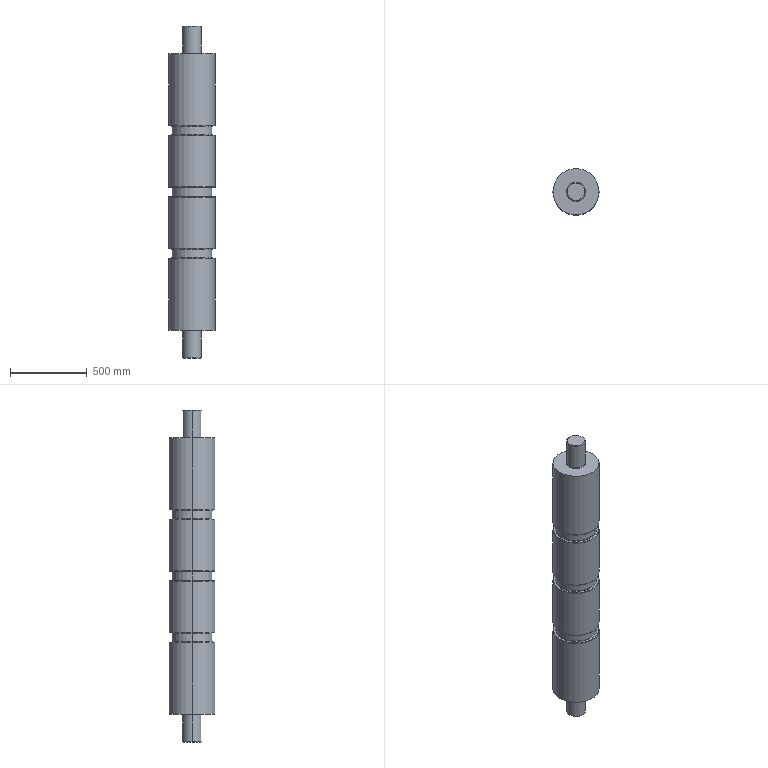Part | SolidWorks | features Chamfer 2, ICE 2, Extrusion 1, Fillet 1, LPattern 1, RefAxis 1, RevCut 1 | 1 solid | 60 faces | box 300 x 300 x 2160 mm | volume 128138036 mm3 | torus 24 | cylinder 18 | plane 10 | cone 8 | commonest cylinder face diameters 300 x8 260 x6 120 x4
STEP:
#1=CARTESIAN_POINT('',(-57.,0.,-180.));
#2=VERTEX_POINT('',#1);
#3=CARTESIAN_POINT('',(57.,0.,-180.));
#4=VERTEX_POINT('',#3);
#5=CARTESIAN_POINT('',(0.,0.,-180.));
#6=DIRECTION('',(0.,0.,-1.));
#7=DIRECTION('',(-1.,0.,0.));
#8=AXIS2_PLACEMENT_3D('',#5,#6,#7);
#9=CIRCLE('',#8,57.);
#10=EDGE_CURVE('',#2,#4,#9,.T.);
#11=ORIENTED_EDGE('',*,*,#10,.F.);
#12=CARTESIAN_POINT('',(-60.,0.,-177.));
#13=VERTEX_POINT('',#12);
#14=CARTESIAN_POINT('',(-57.,0.,-180.));
#15=DIRECTION('',(-0.7071,0.,0.7071));
#16=VECTOR('',#15,1000.);
#17=LINE('',#14,#16);
#18=EDGE_CURVE('',#2,#13,#17,.T.);
#19=ORIENTED_EDGE('',*,*,#18,.T.);
#20=CARTESIAN_POINT('',(60.,0.,-177.));
#21=VERTEX_POINT('',#20);
#22=CARTESIAN_POINT('',(0.,0.,-177.));
#23=DIRECTION('',(0.,0.,1.));
#24=DIRECTION('',(-1.,0.,0.));
#25=AXIS2_PLACEMENT_3D('',#22,#23,#24);
#26=CIRCLE('',#25,60.);
#27=EDGE_CURVE('',#21,#13,#26,.T.);
#28=ORIENTED_EDGE('',*,*,#27,.F.);
#29=CARTESIAN_POINT('',(57.,0.,-180.));
#30=DIRECTION('',(0.7071,0.,0.7071));
#31=VECTOR('',#30,1000.);
#32=LINE('',#29,#31);
#33=EDGE_CURVE('',#4,#21,#32,.T.);
#34=ORIENTED_EDGE('',*,*,#33,.F.);
#35=EDGE_LOOP('',(#11,#19,#28,#34));
#36=FACE_OUTER_BOUND('',#35,.T.);
#37=CARTESIAN_POINT('',(0.,0.,-180.));
#38=DIRECTION('',(0.,0.,1.));
#39=DIRECTION('',(1.,0.,0.));
#40=AXIS2_PLACEMENT_3D('',#37,#38,#39);
#41=CONICAL_SURFACE('',#40,57.,0.7854);
#42=ADVANCED_FACE('',(#36),#41,.T.);
#43=CARTESIAN_POINT('',(-60.,0.,-3.));
#44=VERTEX_POINT('',#43);
#45=CARTESIAN_POINT('',(60.,0.,-3.));
#46=VERTEX_POINT('',#45);
#47=CARTESIAN_POINT('',(0.,0.,-3.));
#48=DIRECTION('',(0.,0.,-1.));
#49=DIRECTION('',(1.,0.,0.));
#50=AXIS2_PLACEMENT_3D('',#47,#48,#49);
#51=CIRCLE('',#50,60.);
#52=EDGE_CURVE('',#44,#46,#51,.T.);
#53=ORIENTED_EDGE('',*,*,#52,.F.);
#54=CARTESIAN_POINT('',(-63.,0.,0.));
#55=VERTEX_POINT('',#54);
#56=CARTESIAN_POINT('',(-60.,0.,-3.));
#57=DIRECTION('',(-0.7071,0.,0.7071));
#58=VECTOR('',#57,1000.);
#59=LINE('',#56,#58);
#60=EDGE_CURVE('',#44,#55,#59,.T.);
#61=ORIENTED_EDGE('',*,*,#60,.T.);
#62=CARTESIAN_POINT('',(63.,0.,0.));
#63=VERTEX_POINT('',#62);
#64=CARTESIAN_POINT('',(0.,0.,0.));
#65=DIRECTION('',(0.,0.,1.));
#66=DIRECTION('',(1.,0.,0.));
#67=AXIS2_PLACEMENT_3D('',#64,#65,#66);
#68=CIRCLE('',#67,63.);
#69=EDGE_CURVE('',#63,#55,#68,.T.);
#70=ORIENTED_EDGE('',*,*,#69,.F.);
#71=CARTESIAN_POINT('',(60.,0.,-3.));
#72=DIRECTION('',(0.7071,0.,0.7071));
#73=VECTOR('',#72,1000.);
#74=LINE('',#71,#73);
#75=EDGE_CURVE('',#46,#63,#74,.T.);
#76=ORIENTED_EDGE('',*,*,#75,.F.);
#77=EDGE_LOOP('',(#53,#61,#70,#76));
#78=FACE_OUTER_BOUND('',#77,.T.);
#79=CARTESIAN_POINT('',(0.,0.,-3.));
#80=DIRECTION('',(0.,0.,1.));
#81=DIRECTION('',(1.,0.,0.));
#82=AXIS2_PLACEMENT_3D('',#79,#80,#81);
#83=CONICAL_SURFACE('',#82,60.,0.7854);
#84=ADVANCED_FACE('',(#78),#83,.T.);
#85=ORIENTED_EDGE('',*,*,#27,.T.);
#86=CARTESIAN_POINT('',(-60.,0.,-180.));
#87=DIRECTION('',(0.,0.,1.));
#88=VECTOR('',#87,1000.);
#89=LINE('',#86,#88);
#90=EDGE_CURVE('',#13,#44,#89,.T.);
#91=ORIENTED_EDGE('',*,*,#90,.T.);
#92=ORIENTED_EDGE('',*,*,#52,.T.);
#93=CARTESIAN_POINT('',(60.,0.,-180.));
#94=DIRECTION('',(0.,0.,1.));
#95=VECTOR('',#94,1000.);
#96=LINE('',#93,#95);
#97=EDGE_CURVE('',#21,#46,#96,.T.);
#98=ORIENTED_EDGE('',*,*,#97,.F.);
#99=EDGE_LOOP('',(#85,#91,#92,#98));
#100=FACE_OUTER_BOUND('',#99,.T.);
#101=CARTESIAN_POINT('',(0.,0.,-180.));
#102=DIRECTION('',(0.,0.,1.));
#103=DIRECTION('',(1.,0.,0.));
#104=AXIS2_PLACEMENT_3D('',#101,#102,#103);
#105=CYLINDRICAL_SURFACE('',#104,60.);
#106=ADVANCED_FACE('',(#100),#105,.T.);
#107=CARTESIAN_POINT('',(57.,0.,1980.));
#108=VERTEX_POINT('',#107);
#109=CARTESIAN_POINT('',(-57.,0.,1980.));
#110=VERTEX_POINT('',#109);
#111=CARTESIAN_POINT('',(0.,0.,1980.));
#112=DIRECTION('',(0.,0.,1.));
#113=DIRECTION('',(1.,0.,0.));
#114=AXIS2_PLACEMENT_3D('',#111,#112,#113);
#115=CIRCLE('',#114,57.);
#116=EDGE_CURVE('',#108,#110,#115,.T.);
#117=ORIENTED_EDGE('',*,*,#116,.F.);
#118=CARTESIAN_POINT('',(60.,0.,1977.));
#119=VERTEX_POINT('',#118);
#120=CARTESIAN_POINT('',(57.,0.,1980.));
#121=DIRECTION('',(0.7071,0.,-0.7071));
#122=VECTOR('',#121,1000.);
#123=LINE('',#120,#122);
#124=EDGE_CURVE('',#108,#119,#123,.T.);
#125=ORIENTED_EDGE('',*,*,#124,.T.);
#126=CARTESIAN_POINT('',(-60.,0.,1977.));
#127=VERTEX_POINT('',#126);
#128=CARTESIAN_POINT('',(0.,0.,1977.));
#129=DIRECTION('',(0.,0.,-1.));
#130=DIRECTION('',(1.,0.,0.));
#131=AXIS2_PLACEMENT_3D('',#128,#129,#130);
#132=CIRCLE('',#131,60.);
#133=EDGE_CURVE('',#127,#119,#132,.T.);
#134=ORIENTED_EDGE('',*,*,#133,.F.);
#135=CARTESIAN_POINT('',(-57.,0.,1980.));
#136=DIRECTION('',(-0.7071,0.,-0.7071));
#137=VECTOR('',#136,1000.);
#138=LINE('',#135,#137);
#139=EDGE_CURVE('',#110,#127,#138,.T.);
#140=ORIENTED_EDGE('',*,*,#139,.F.);
#141=EDGE_LOOP('',(#117,#125,#134,#140));
#142=FACE_OUTER_BOUND('',#141,.T.);
#143=CARTESIAN_POINT('',(0.,0.,1980.));
#144=DIRECTION('',(0.,0.,-1.));
#145=DIRECTION('',(-1.,0.,0.));
#146=AXIS2_PLACEMENT_3D('',#143,#144,#145);
#147=CONICAL_SURFACE('',#146,57.,0.7854);
#148=ADVANCED_FACE('',(#142),#147,.T.);
#149=CARTESIAN_POINT('',(60.,0.,1803.));
#150=VERTEX_POINT('',#149);
#151=CARTESIAN_POINT('',(-60.,0.,1803.));
#152=VERTEX_POINT('',#151);
#153=CARTESIAN_POINT('',(0.,0.,1803.));
#154=DIRECTION('',(0.,0.,1.));
#155=DIRECTION('',(1.,0.,0.));
#156=AXIS2_PLACEMENT_3D('',#153,#154,#155);
#157=CIRCLE('',#156,60.);
#158=EDGE_CURVE('',#150,#152,#157,.T.);
#159=ORIENTED_EDGE('',*,*,#158,.F.);
#160=CARTESIAN_POINT('',(63.,0.,1800.));
#161=VERTEX_POINT('',#160);
#162=CARTESIAN_POINT('',(60.,0.,1803.));
#163=DIRECTION('',(0.7071,0.,-0.7071));
#164=VECTOR('',#163,1000.);
#165=LINE('',#162,#164);
#166=EDGE_CURVE('',#150,#161,#165,.T.);
#167=ORIENTED_EDGE('',*,*,#166,.T.);
#168=CARTESIAN_POINT('',(-63.,0.,1800.));
#169=VERTEX_POINT('',#168);
#170=CARTESIAN_POINT('',(0.,0.,1800.));
#171=DIRECTION('',(0.,0.,-1.));
#172=DIRECTION('',(1.,0.,0.));
#173=AXIS2_PLACEMENT_3D('',#170,#171,#172);
#174=CIRCLE('',#173,63.);
#175=EDGE_CURVE('',#169,#161,#174,.T.);
#176=ORIENTED_EDGE('',*,*,#175,.F.);
#177=CARTESIAN_POINT('',(-60.,0.,1803.));
#178=DIRECTION('',(-0.7071,0.,-0.7071));
#179=VECTOR('',#178,1000.);
#180=LINE('',#177,#179);
#181=EDGE_CURVE('',#152,#169,#180,.T.);
#182=ORIENTED_EDGE('',*,*,#181,.F.);
#183=EDGE_LOOP('',(#159,#167,#176,#182));
#184=FACE_OUTER_BOUND('',#183,.T.);
#185=CARTESIAN_POINT('',(0.,0.,1803.));
#186=DIRECTION('',(0.,0.,-1.));
#187=DIRECTION('',(-1.,0.,0.));
#188=AXIS2_PLACEMENT_3D('',#185,#186,#187);
#189=CONICAL_SURFACE('',#188,60.,0.7854);
#190=ADVANCED_FACE('',(#184),#189,.T.);
#191=ORIENTED_EDGE('',*,*,#133,.T.);
#192=CARTESIAN_POINT('',(60.,0.,1980.));
#193=DIRECTION('',(0.,0.,-1.));
#194=VECTOR('',#193,1000.);
#195=LINE('',#192,#194);
#196=EDGE_CURVE('',#119,#150,#195,.T.);
#197=ORIENTED_EDGE('',*,*,#196,.T.);
#198=ORIENTED_EDGE('',*,*,#158,.T.);
#199=CARTESIAN_POINT('',(-60.,0.,1980.));
#200=DIRECTION('',(0.,0.,-1.));
#201=VECTOR('',#200,1000.);
#202=LINE('',#199,#201);
#203=EDGE_CURVE('',#127,#152,#202,.T.);
#204=ORIENTED_EDGE('',*,*,#203,.F.);
#205=EDGE_LOOP('',(#191,#197,#198,#204));
#206=FACE_OUTER_BOUND('',#205,.T.);
#207=CARTESIAN_POINT('',(0.,0.,1980.));
#208=DIRECTION('',(0.,0.,-1.));
#209=DIRECTION('',(-1.,0.,0.));
#210=AXIS2_PLACEMENT_3D('',#207,#208,#209);
#211=CYLINDRICAL_SURFACE('',#210,60.);
#212=ADVANCED_FACE('',(#206),#211,.T.);
#213=CARTESIAN_POINT('',(-130.,0.,473.));
#214=VERTEX_POINT('',#213);
#215=CARTESIAN_POINT('',(130.,0.,473.));
#216=VERTEX_POINT('',#215);
#217=CARTESIAN_POINT('',(0.,0.,473.));
#218=DIRECTION('',(0.,0.,1.));
#219=DIRECTION('',(1.,0.,0.));
#220=AXIS2_PLACEMENT_3D('',#217,#218,#219);
#221=CIRCLE('',#220,130.);
#222=EDGE_CURVE('',#214,#216,#221,.T.);
#223=ORIENTED_EDGE('',*,*,#222,.F.);
#224=CARTESIAN_POINT('',(-133.,0.,470.));
#225=VERTEX_POINT('',#224);
#226=CARTESIAN_POINT('',(-133.,0.,473.));
#227=DIRECTION('',(0.,1.,0.));
#228=DIRECTION('',(-1.,0.,0.));
#229=AXIS2_PLACEMENT_3D('',#226,#227,#228);
#230=CIRCLE('',#229,3.);
#231=EDGE_CURVE('',#214,#225,#230,.T.);
#232=ORIENTED_EDGE('',*,*,#231,.T.);
#233=CARTESIAN_POINT('',(133.,0.,470.));
#234=VERTEX_POINT('',#233);
#235=CARTESIAN_POINT('',(0.,0.,470.));
#236=DIRECTION('',(0.,0.,-1.));
#237=DIRECTION('',(1.,0.,0.));
#238=AXIS2_PLACEMENT_3D('',#235,#236,#237);
#239=CIRCLE('',#238,133.);
#240=EDGE_CURVE('',#234,#225,#239,.T.);
#241=ORIENTED_EDGE('',*,*,#240,.F.);
#242=CARTESIAN_POINT('',(133.,0.,473.));
#243=DIRECTION('',(0.,-1.,0.));
#244=DIRECTION('',(0.,0.,-1.));
#245=AXIS2_PLACEMENT_3D('',#242,#243,#244);
#246=CIRCLE('',#245,3.);
#247=EDGE_CURVE('',#216,#234,#246,.T.);
#248=ORIENTED_EDGE('',*,*,#247,.F.);
#249=EDGE_LOOP('',(#223,#232,#241,#248));
#250=FACE_OUTER_BOUND('',#249,.T.);
#251=CARTESIAN_POINT('',(0.,0.,473.));
#252=DIRECTION('',(0.,0.,1.));
#253=DIRECTION('',(1.,0.,0.));
#254=AXIS2_PLACEMENT_3D('',#251,#252,#253);
#255=TOROIDAL_SURFACE('',#254,133.,3.);
#256=ADVANCED_FACE('',(#250),#255,.F.);
#257=CARTESIAN_POINT('',(-150.,0.,467.));
#258=VERTEX_POINT('',#257);
#259=CARTESIAN_POINT('',(150.,0.,467.));
#260=VERTEX_POINT('',#259);
#261=CARTESIAN_POINT('',(0.,0.,467.));
#262=DIRECTION('',(0.,0.,-1.));
#263=DIRECTION('',(1.,0.,0.));
#264=AXIS2_PLACEMENT_3D('',#261,#262,#263);
#265=CIRCLE('',#264,150.);
#266=EDGE_CURVE('',#258,#260,#265,.T.);
#267=ORIENTED_EDGE('',*,*,#266,.F.);
#268=CARTESIAN_POINT('',(-147.,0.,470.));
#269=VERTEX_POINT('',#268);
#270=CARTESIAN_POINT('',(-147.,0.,467.));
#271=DIRECTION('',(0.,1.,0.));
#272=DIRECTION('',(-1.,0.,0.));
#273=AXIS2_PLACEMENT_3D('',#270,#271,#272);
#274=CIRCLE('',#273,3.);
#275=EDGE_CURVE('',#258,#269,#274,.T.);
#276=ORIENTED_EDGE('',*,*,#275,.T.);
#277=CARTESIAN_POINT('',(147.,0.,470.));
#278=VERTEX_POINT('',#277);
#279=CARTESIAN_POINT('',(0.,0.,470.));
#280=DIRECTION('',(0.,0.,1.));
#281=DIRECTION('',(1.,0.,0.));
#282=AXIS2_PLACEMENT_3D('',#279,#280,#281);
#283=CIRCLE('',#282,147.);
#284=EDGE_CURVE('',#278,#269,#283,.T.);
#285=ORIENTED_EDGE('',*,*,#284,.F.);
#286=CARTESIAN_POINT('',(147.,0.,467.));
#287=DIRECTION('',(0.,-1.,0.));
#288=DIRECTION('',(0.,0.,-1.));
#289=AXIS2_PLACEMENT_3D('',#286,#287,#288);
#290=CIRCLE('',#289,3.);
#291=EDGE_CURVE('',#260,#278,#290,.T.);
#292=ORIENTED_EDGE('',*,*,#291,.F.);
#293=EDGE_LOOP('',(#267,#276,#285,#292));
#294=FACE_OUTER_BOUND('',#293,.T.);
#295=CARTESIAN_POINT('',(0.,0.,467.));
#296=DIRECTION('',(0.,0.,1.));
#297=DIRECTION('',(1.,0.,0.));
#298=AXIS2_PLACEMENT_3D('',#295,#296,#297);
#299=TOROIDAL_SURFACE('',#298,147.,3.);
#300=ADVANCED_FACE('',(#294),#299,.T.);
#301=CARTESIAN_POINT('',(150.,0.,533.));
#302=VERTEX_POINT('',#301);
#303=CARTESIAN_POINT('',(-150.,0.,533.));
#304=VERTEX_POINT('',#303);
#305=CARTESIAN_POINT('',(0.,0.,533.));
#306=DIRECTION('',(0.,0.,1.));
#307=DIRECTION('',(-1.,0.,0.));
#308=AXIS2_PLACEMENT_3D('',#305,#306,#307);
#309=CIRCLE('',#308,150.);
#310=EDGE_CURVE('',#302,#304,#309,.T.);
#311=ORIENTED_EDGE('',*,*,#310,.F.);
#312=CARTESIAN_POINT('',(147.,0.,530.));
#313=VERTEX_POINT('',#312);
#314=CARTESIAN_POINT('',(147.,0.,533.));
#315=DIRECTION('',(0.,1.,0.));
#316=DIRECTION('',(-1.,0.,0.));
#317=AXIS2_PLACEMENT_3D('',#314,#315,#316);
#318=CIRCLE('',#317,3.);
#319=EDGE_CURVE('',#302,#313,#318,.T.);
#320=ORIENTED_EDGE('',*,*,#319,.T.);
#321=CARTESIAN_POINT('',(-147.,0.,530.));
#322=VERTEX_POINT('',#321);
#323=CARTESIAN_POINT('',(0.,0.,530.));
#324=DIRECTION('',(0.,0.,-1.));
#325=DIRECTION('',(-1.,0.,0.));
#326=AXIS2_PLACEMENT_3D('',#323,#324,#325);
#327=CIRCLE('',#326,147.);
#328=EDGE_CURVE('',#322,#313,#327,.T.);
#329=ORIENTED_EDGE('',*,*,#328,.F.);
#330=CARTESIAN_POINT('',(-147.,0.,533.));
#331=DIRECTION('',(0.,-1.,0.));
#332=DIRECTION('',(0.,0.,-1.));
#333=AXIS2_PLACEMENT_3D('',#330,#331,#332);
#334=CIRCLE('',#333,3.);
#335=EDGE_CURVE('',#304,#322,#334,.T.);
#336=ORIENTED_EDGE('',*,*,#335,.F.);
#337=EDGE_LOOP('',(#311,#320,#329,#336));
#338=FACE_OUTER_BOUND('',#337,.T.);
#339=CARTESIAN_POINT('',(0.,0.,533.));
#340=DIRECTION('',(0.,0.,-1.));
#341=DIRECTION('',(-1.,0.,0.));
#342=AXIS2_PLACEMENT_3D('',#339,#340,#341);
#343=TOROIDAL_SURFACE('',#342,147.,3.);
#344=ADVANCED_FACE('',(#338),#343,.T.);
#345=CARTESIAN_POINT('',(130.,0.,527.));
#346=VERTEX_POINT('',#345);
#347=CARTESIAN_POINT('',(-130.,0.,527.));
#348=VERTEX_POINT('',#347);
#349=CARTESIAN_POINT('',(0.,0.,527.));
#350=DIRECTION('',(0.,0.,-1.));
#351=DIRECTION('',(-1.,0.,0.));
#352=AXIS2_PLACEMENT_3D('',#349,#350,#351);
#353=CIRCLE('',#352,130.);
#354=EDGE_CURVE('',#346,#348,#353,.T.);
#355=ORIENTED_EDGE('',*,*,#354,.F.);
#356=CARTESIAN_POINT('',(133.,0.,530.));
#357=VERTEX_POINT('',#356);
#358=CARTESIAN_POINT('',(133.,0.,527.));
#359=DIRECTION('',(0.,1.,0.));
#360=DIRECTION('',(-1.,0.,0.));
#361=AXIS2_PLACEMENT_3D('',#358,#359,#360);
#362=CIRCLE('',#361,3.);
#363=EDGE_CURVE('',#346,#357,#362,.T.);
#364=ORIENTED_EDGE('',*,*,#363,.T.);
#365=CARTESIAN_POINT('',(-133.,0.,530.));
#366=VERTEX_POINT('',#365);
#367=CARTESIAN_POINT('',(0.,0.,530.));
#368=DIRECTION('',(0.,0.,1.));
#369=DIRECTION('',(-1.,0.,0.));
#370=AXIS2_PLACEMENT_3D('',#367,#368,#369);
#371=CIRCLE('',#370,133.);
#372=EDGE_CURVE('',#366,#357,#371,.T.);
#373=ORIENTED_EDGE('',*,*,#372,.F.);
#374=CARTESIAN_POINT('',(-133.,0.,527.));
#375=DIRECTION('',(0.,-1.,0.));
#376=DIRECTION('',(0.,0.,-1.));
#377=AXIS2_PLACEMENT_3D('',#374,#375,#376);
#378=CIRCLE('',#377,3.);
#379=EDGE_CURVE('',#348,#366,#378,.T.);
#380=ORIENTED_EDGE('',*,*,#379,.F.);
#381=EDGE_LOOP('',(#355,#364,#373,#380));
#382=FACE_OUTER_BOUND('',#381,.T.);
#383=CARTESIAN_POINT('',(0.,0.,527.));
#384=DIRECTION('',(0.,0.,-1.));
#385=DIRECTION('',(-1.,0.,0.));
#386=AXIS2_PLACEMENT_3D('',#383,#384,#385);
#387=TOROIDAL_SURFACE('',#386,133.,3.);
#388=ADVANCED_FACE('',(#382),#387,.F.);
#389=CARTESIAN_POINT('',(-130.,0.,1273.));
#390=VERTEX_POINT('',#389);
#391=CARTESIAN_POINT('',(130.,0.,1273.));
#392=VERTEX_POINT('',#391);
#393=CARTESIAN_POINT('',(0.,0.,1273.));
#394=DIRECTION('',(0.,0.,1.));
#395=DIRECTION('',(1.,0.,0.));
#396=AXIS2_PLACEMENT_3D('',#393,#394,#395);
#397=CIRCLE('',#396,130.);
#398=EDGE_CURVE('',#390,#392,#397,.T.);
#399=ORIENTED_EDGE('',*,*,#398,.F.);
#400=CARTESIAN_POINT('',(-133.,0.,1270.));
#401=VERTEX_POINT('',#400);
#402=CARTESIAN_POINT('',(-133.,0.,1273.));
#403=DIRECTION('',(0.,1.,0.));
#404=DIRECTION('',(-1.,0.,0.));
#405=AXIS2_PLACEMENT_3D('',#402,#403,#404);
#406=CIRCLE('',#405,3.);
#407=EDGE_CURVE('',#390,#401,#406,.T.);
#408=ORIENTED_EDGE('',*,*,#407,.T.);
#409=CARTESIAN_POINT('',(133.,0.,1270.));
#410=VERTEX_POINT('',#409);
#411=CARTESIAN_POINT('',(0.,0.,1270.));
#412=DIRECTION('',(0.,0.,-1.));
#413=DIRECTION('',(1.,0.,0.));
#414=AXIS2_PLACEMENT_3D('',#411,#412,#413);
#415=CIRCLE('',#414,133.);
#416=EDGE_CURVE('',#410,#401,#415,.T.);
#417=ORIENTED_EDGE('',*,*,#416,.F.);
#418=CARTESIAN_POINT('',(133.,0.,1273.));
#419=DIRECTION('',(0.,-1.,0.));
#420=DIRECTION('',(0.,0.,-1.));
#421=AXIS2_PLACEMENT_3D('',#418,#419,#420);
#422=CIRCLE('',#421,3.);
#423=EDGE_CURVE('',#392,#410,#422,.T.);
#424=ORIENTED_EDGE('',*,*,#423,.F.);
#425=EDGE_LOOP('',(#399,#408,#417,#424));
#426=FACE_OUTER_BOUND('',#425,.T.);
#427=CARTESIAN_POINT('',(0.,0.,1273.));
#428=DIRECTION('',(0.,0.,1.));
#429=DIRECTION('',(1.,0.,0.));
#430=AXIS2_PLACEMENT_3D('',#427,#428,#429);
#431=TOROIDAL_SURFACE('',#430,133.,3.);
#432=ADVANCED_FACE('',(#426),#431,.F.);
#433=CARTESIAN_POINT('',(-150.,0.,1267.));
#434=VERTEX_POINT('',#433);
#435=CARTESIAN_POINT('',(150.,0.,1267.));
#436=VERTEX_POINT('',#435);
#437=CARTESIAN_POINT('',(0.,0.,1267.));
#438=DIRECTION('',(0.,0.,-1.));
#439=DIRECTION('',(1.,0.,0.));
#440=AXIS2_PLACEMENT_3D('',#437,#438,#439);
#441=CIRCLE('',#440,150.);
#442=EDGE_CURVE('',#434,#436,#441,.T.);
#443=ORIENTED_EDGE('',*,*,#442,.F.);
#444=CARTESIAN_POINT('',(-147.,0.,1270.));
#445=VERTEX_POINT('',#444);
#446=CARTESIAN_POINT('',(-147.,0.,1267.));
#447=DIRECTION('',(0.,1.,0.));
#448=DIRECTION('',(-1.,0.,0.));
#449=AXIS2_PLACEMENT_3D('',#446,#447,#448);
#450=CIRCLE('',#449,3.);
#451=EDGE_CURVE('',#434,#445,#450,.T.);
#452=ORIENTED_EDGE('',*,*,#451,.T.);
#453=CARTESIAN_POINT('',(147.,0.,1270.));
#454=VERTEX_POINT('',#453);
#455=CARTESIAN_POINT('',(0.,0.,1270.));
#456=DIRECTION('',(0.,0.,1.));
#457=DIRECTION('',(1.,0.,0.));
#458=AXIS2_PLACEMENT_3D('',#455,#456,#457);
#459=CIRCLE('',#458,147.);
#460=EDGE_CURVE('',#454,#445,#459,.T.);
#461=ORIENTED_EDGE('',*,*,#460,.F.);
#462=CARTESIAN_POINT('',(147.,0.,1267.));
#463=DIRECTION('',(0.,-1.,0.));
#464=DIRECTION('',(0.,0.,-1.));
#465=AXIS2_PLACEMENT_3D('',#462,#463,#464);
#466=CIRCLE('',#465,3.);
#467=EDGE_CURVE('',#436,#454,#466,.T.);
#468=ORIENTED_EDGE('',*,*,#467,.F.);
#469=EDGE_LOOP('',(#443,#452,#461,#468));
#470=FACE_OUTER_BOUND('',#469,.T.);
#471=CARTESIAN_POINT('',(0.,0.,1267.));
#472=DIRECTION('',(0.,0.,1.));
#473=DIRECTION('',(1.,0.,0.));
#474=AXIS2_PLACEMENT_3D('',#471,#472,#473);
#475=TOROIDAL_SURFACE('',#474,147.,3.);
#476=ADVANCED_FACE('',(#470),#475,.T.);
#477=CARTESIAN_POINT('',(150.,0.,1333.));
#478=VERTEX_POINT('',#477);
#479=CARTESIAN_POINT('',(-150.,0.,1333.));
#480=VERTEX_POINT('',#479);
#481=CARTESIAN_POINT('',(0.,0.,1333.));
#482=DIRECTION('',(0.,0.,1.));
#483=DIRECTION('',(-1.,0.,0.));
#484=AXIS2_PLACEMENT_3D('',#481,#482,#483);
#485=CIRCLE('',#484,150.);
#486=EDGE_CURVE('',#478,#480,#485,.T.);
#487=ORIENTED_EDGE('',*,*,#486,.F.);
#488=CARTESIAN_POINT('',(147.,0.,1330.));
#489=VERTEX_POINT('',#488);
#490=CARTESIAN_POINT('',(147.,0.,1333.));
#491=DIRECTION('',(0.,1.,0.));
#492=DIRECTION('',(-1.,0.,0.));
#493=AXIS2_PLACEMENT_3D('',#490,#491,#492);
#494=CIRCLE('',#493,3.);
#495=EDGE_CURVE('',#478,#489,#494,.T.);
#496=ORIENTED_EDGE('',*,*,#495,.T.);
#497=CARTESIAN_POINT('',(-147.,0.,1330.));
#498=VERTEX_POINT('',#497);
#499=CARTESIAN_POINT('',(0.,0.,1330.));
#500=DIRECTION('',(0.,0.,-1.));
#501=DIRECTION('',(-1.,0.,0.));
#502=AXIS2_PLACEMENT_3D('',#499,#500,#501);
#503=CIRCLE('',#502,147.);
#504=EDGE_CURVE('',#498,#489,#503,.T.);
#505=ORIENTED_EDGE('',*,*,#504,.F.);
#506=CARTESIAN_POINT('',(-147.,0.,1333.));
#507=DIRECTION('',(0.,-1.,0.));
#508=DIRECTION('',(0.,0.,-1.));
#509=AXIS2_PLACEMENT_3D('',#506,#507,#508);
#510=CIRCLE('',#509,3.);
#511=EDGE_CURVE('',#480,#498,#510,.T.);
#512=ORIENTED_EDGE('',*,*,#511,.F.);
#513=EDGE_LOOP('',(#487,#496,#505,#512));
#514=FACE_OUTER_BOUND('',#513,.T.);
#515=CARTESIAN_POINT('',(0.,0.,1333.));
#516=DIRECTION('',(0.,0.,-1.));
#517=DIRECTION('',(-1.,0.,0.));
#518=AXIS2_PLACEMENT_3D('',#515,#516,#517);
#519=TOROIDAL_SURFACE('',#518,147.,3.);
#520=ADVANCED_FACE('',(#514),#519,.T.);
#521=CARTESIAN_POINT('',(130.,0.,1327.));
#522=VERTEX_POINT('',#521);
#523=CARTESIAN_POINT('',(-130.,0.,1327.));
#524=VERTEX_POINT('',#523);
#525=CARTESIAN_POINT('',(0.,0.,1327.));
#526=DIRECTION('',(0.,0.,-1.));
#527=DIRECTION('',(-1.,0.,0.));
#528=AXIS2_PLACEMENT_3D('',#525,#526,#527);
#529=CIRCLE('',#528,130.);
#530=EDGE_CURVE('',#522,#524,#529,.T.);
#531=ORIENTED_EDGE('',*,*,#530,.F.);
#532=CARTESIAN_POINT('',(133.,0.,1330.));
#533=VERTEX_POINT('',#532);
#534=CARTESIAN_POINT('',(133.,0.,1327.));
#535=DIRECTION('',(0.,1.,0.));
#536=DIRECTION('',(-1.,0.,0.));
#537=AXIS2_PLACEMENT_3D('',#534,#535,#536);
#538=CIRCLE('',#537,3.);
#539=EDGE_CURVE('',#522,#533,#538,.T.);
#540=ORIENTED_EDGE('',*,*,#539,.T.);
#541=CARTESIAN_POINT('',(-133.,0.,1330.));
#542=VERTEX_POINT('',#541);
#543=CARTESIAN_POINT('',(0.,0.,1330.));
#544=DIRECTION('',(0.,0.,1.));
#545=DIRECTION('',(-1.,0.,0.));
#546=AXIS2_PLACEMENT_3D('',#543,#544,#545);
#547=CIRCLE('',#546,133.);
#548=EDGE_CURVE('',#542,#533,#547,.T.);
#549=ORIENTED_EDGE('',*,*,#548,.F.);
#550=CARTESIAN_POINT('',(-133.,0.,1327.));
#551=DIRECTION('',(0.,-1.,0.));
#552=DIRECTION('',(0.,0.,-1.));
#553=AXIS2_PLACEMENT_3D('',#550,#551,#552);
#554=CIRCLE('',#553,3.);
#555=EDGE_CURVE('',#524,#542,#554,.T.);
#556=ORIENTED_EDGE('',*,*,#555,.F.);
#557=EDGE_LOOP('',(#531,#540,#549,#556));
#558=FACE_OUTER_BOUND('',#557,.T.);
#559=CARTESIAN_POINT('',(0.,0.,1327.));
#560=DIRECTION('',(0.,0.,-1.));
#561=DIRECTION('',(-1.,0.,0.));
#562=AXIS2_PLACEMENT_3D('',#559,#560,#561);
#563=TOROIDAL_SURFACE('',#562,133.,3.);
#564=ADVANCED_FACE('',(#558),#563,.F.);
#565=ORIENTED_EDGE('',*,*,#266,.T.);
#566=CARTESIAN_POINT('',(150.,0.,0.));
#567=VERTEX_POINT('',#566);
#568=CARTESIAN_POINT('',(150.,0.,1800.));
#569=DIRECTION('',(0.,0.,-1.));
#570=VECTOR('',#569,1000.);
#571=LINE('',#568,#570);
#572=EDGE_CURVE('',#260,#567,#571,.T.);
#573=ORIENTED_EDGE('',*,*,#572,.T.);
#574=CARTESIAN_POINT('',(-150.,0.,0.));
#575=VERTEX_POINT('',#574);
#576=CARTESIAN_POINT('',(0.,0.,0.));
#577=DIRECTION('',(0.,0.,1.));
#578=DIRECTION('',(1.,0.,0.));
#579=AXIS2_PLACEMENT_3D('',#576,#577,#578);
#580=CIRCLE('',#579,150.);
#581=EDGE_CURVE('',#567,#575,#580,.T.);
#582=ORIENTED_EDGE('',*,*,#581,.T.);
#583=CARTESIAN_POINT('',(-150.,0.,1800.));
#584=DIRECTION('',(0.,0.,-1.));
#585=VECTOR('',#584,1000.);
#586=LINE('',#583,#585);
#587=EDGE_CURVE('',#258,#575,#586,.T.);
#588=ORIENTED_EDGE('',*,*,#587,.F.);
#589=EDGE_LOOP('',(#565,#573,#582,#588));
#590=FACE_OUTER_BOUND('',#589,.T.);
#591=CARTESIAN_POINT('',(0.,0.,1800.));
#592=DIRECTION('',(0.,0.,-1.));
#593=DIRECTION('',(-1.,0.,0.));
#594=AXIS2_PLACEMENT_3D('',#591,#592,#593);
#595=CYLINDRICAL_SURFACE('',#594,150.);
#596=ADVANCED_FACE('',(#590),#595,.T.);
#597=CARTESIAN_POINT('',(0.,0.,527.));
#598=DIRECTION('',(0.,0.,-1.));
#599=DIRECTION('',(-1.,0.,0.));
#600=AXIS2_PLACEMENT_3D('',#597,#598,#599);
#601=CIRCLE('',#600,130.);
#602=EDGE_CURVE('',#348,#346,#601,.T.);
#603=ORIENTED_EDGE('',*,*,#602,.T.);
#604=CARTESIAN_POINT('',(130.,0.,-400.));
#605=DIRECTION('',(0.,0.,-1.));
#606=VECTOR('',#605,1000.);
#607=LINE('',#604,#606);
#608=EDGE_CURVE('',#346,#216,#607,.T.);
#609=ORIENTED_EDGE('',*,*,#608,.T.);
#610=CARTESIAN_POINT('',(0.,0.,473.));
#611=DIRECTION('',(0.,0.,1.));
#612=DIRECTION('',(1.,0.,0.));
#613=AXIS2_PLACEMENT_3D('',#610,#611,#612);
#614=CIRCLE('',#613,130.);
#615=EDGE_CURVE('',#216,#214,#614,.T.);
#616=ORIENTED_EDGE('',*,*,#615,.T.);
#617=CARTESIAN_POINT('',(-130.,0.,-400.));
#618=DIRECTION('',(0.,0.,-1.));
#619=VECTOR('',#618,1000.);
#620=LINE('',#617,#619);
#621=EDGE_CURVE('',#348,#214,#620,.T.);
#622=ORIENTED_EDGE('',*,*,#621,.F.);
#623=EDGE_LOOP('',(#603,#609,#616,#622));
#624=FACE_OUTER_BOUND('',#623,.T.);
#625=CARTESIAN_POINT('',(0.,0.,-400.));
#626=DIRECTION('',(0.,0.,-1.));
#627=DIRECTION('',(-1.,0.,0.));
#628=AXIS2_PLACEMENT_3D('',#625,#626,#627);
#629=CYLINDRICAL_SURFACE('',#628,130.);
#630=ADVANCED_FACE('',(#624),#629,.T.);
#631=CARTESIAN_POINT('',(150.,0.,1800.));
#632=VERTEX_POINT('',#631);
#633=CARTESIAN_POINT('',(-150.,0.,1800.));
#634=VERTEX_POINT('',#633);
#635=CARTESIAN_POINT('',(0.,0.,1800.));
#636=DIRECTION('',(0.,0.,1.));
#637=DIRECTION('',(1.,0.,0.));
#638=AXIS2_PLACEMENT_3D('',#635,#636,#637);
#639=CIRCLE('',#638,150.);
#640=EDGE_CURVE('',#632,#634,#639,.T.);
#641=ORIENTED_EDGE('',*,*,#640,.F.);
#642=CARTESIAN_POINT('',(150.,0.,1800.));
#643=DIRECTION('',(0.,0.,-1.));
#644=VECTOR('',#643,1000.);
#645=LINE('',#642,#644);
#646=EDGE_CURVE('',#632,#478,#645,.T.);
#647=ORIENTED_EDGE('',*,*,#646,.T.);
#648=ORIENTED_EDGE('',*,*,#486,.T.);
#649=CARTESIAN_POINT('',(-150.,0.,1800.));
#650=DIRECTION('',(0.,0.,-1.));
#651=VECTOR('',#650,1000.);
#652=LINE('',#649,#651);
#653=EDGE_CURVE('',#634,#480,#652,.T.);
#654=ORIENTED_EDGE('',*,*,#653,.F.);
#655=EDGE_LOOP('',(#641,#647,#648,#654));
#656=FACE_OUTER_BOUND('',#655,.T.);
#657=CARTESIAN_POINT('',(0.,0.,1800.));
#658=DIRECTION('',(0.,0.,-1.));
#659=DIRECTION('',(-1.,0.,0.));
#660=AXIS2_PLACEMENT_3D('',#657,#658,#659);
#661=CYLINDRICAL_SURFACE('',#660,150.);
#662=ADVANCED_FACE('',(#656),#661,.T.);
#663=CARTESIAN_POINT('',(0.,0.,1327.));
#664=DIRECTION('',(0.,0.,-1.));
#665=DIRECTION('',(-1.,0.,0.));
#666=AXIS2_PLACEMENT_3D('',#663,#664,#665);
#667=CIRCLE('',#666,130.);
#668=EDGE_CURVE('',#524,#522,#667,.T.);
#669=ORIENTED_EDGE('',*,*,#668,.T.);
#670=CARTESIAN_POINT('',(130.,0.,400.));
#671=DIRECTION('',(0.,0.,-1.));
#672=VECTOR('',#671,1000.);
#673=LINE('',#670,#672);
#674=EDGE_CURVE('',#522,#392,#673,.T.);
#675=ORIENTED_EDGE('',*,*,#674,.T.);
#676=CARTESIAN_POINT('',(0.,0.,1273.));
#677=DIRECTION('',(0.,0.,1.));
#678=DIRECTION('',(1.,0.,0.));
#679=AXIS2_PLACEMENT_3D('',#676,#677,#678);
#680=CIRCLE('',#679,130.);
#681=EDGE_CURVE('',#392,#390,#680,.T.);
#682=ORIENTED_EDGE('',*,*,#681,.T.);
#683=CARTESIAN_POINT('',(-130.,0.,400.));
#684=DIRECTION('',(0.,0.,-1.));
#685=VECTOR('',#684,1000.);
#686=LINE('',#683,#685);
#687=EDGE_CURVE('',#524,#390,#686,.T.);
#688=ORIENTED_EDGE('',*,*,#687,.F.);
#689=EDGE_LOOP('',(#669,#675,#682,#688));
#690=FACE_OUTER_BOUND('',#689,.T.);
#691=CARTESIAN_POINT('',(0.,0.,400.));
#692=DIRECTION('',(0.,0.,-1.));
#693=DIRECTION('',(-1.,0.,0.));
#694=AXIS2_PLACEMENT_3D('',#691,#692,#693);
#695=CYLINDRICAL_SURFACE('',#694,130.);
#696=ADVANCED_FACE('',(#690),#695,.T.);
#697=CARTESIAN_POINT('',(-130.,0.,873.));
#698=VERTEX_POINT('',#697);
#699=CARTESIAN_POINT('',(130.,0.,873.));
#700=VERTEX_POINT('',#699);
#701=CARTESIAN_POINT('',(0.,0.,873.));
#702=DIRECTION('',(0.,0.,1.));
#703=DIRECTION('',(1.,0.,0.));
#704=AXIS2_PLACEMENT_3D('',#701,#702,#703);
#705=CIRCLE('',#704,130.);
#706=EDGE_CURVE('',#698,#700,#705,.T.);
#707=ORIENTED_EDGE('',*,*,#706,.F.);
#708=CARTESIAN_POINT('',(-133.,0.,870.));
#709=VERTEX_POINT('',#708);
#710=CARTESIAN_POINT('',(-133.,0.,873.));
#711=DIRECTION('',(0.,1.,0.));
#712=DIRECTION('',(-1.,0.,0.));
#713=AXIS2_PLACEMENT_3D('',#710,#711,#712);
#714=CIRCLE('',#713,3.);
#715=EDGE_CURVE('',#698,#709,#714,.T.);
#716=ORIENTED_EDGE('',*,*,#715,.T.);
#717=CARTESIAN_POINT('',(133.,0.,870.));
#718=VERTEX_POINT('',#717);
#719=CARTESIAN_POINT('',(0.,0.,870.));
#720=DIRECTION('',(0.,0.,-1.));
#721=DIRECTION('',(1.,0.,0.));
#722=AXIS2_PLACEMENT_3D('',#719,#720,#721);
#723=CIRCLE('',#722,133.);
#724=EDGE_CURVE('',#718,#709,#723,.T.);
#725=ORIENTED_EDGE('',*,*,#724,.F.);
#726=CARTESIAN_POINT('',(133.,0.,873.));
#727=DIRECTION('',(0.,-1.,0.));
#728=DIRECTION('',(0.,0.,-1.));
#729=AXIS2_PLACEMENT_3D('',#726,#727,#728);
#730=CIRCLE('',#729,3.);
#731=EDGE_CURVE('',#700,#718,#730,.T.);
#732=ORIENTED_EDGE('',*,*,#731,.F.);
#733=EDGE_LOOP('',(#707,#716,#725,#732));
#734=FACE_OUTER_BOUND('',#733,.T.);
#735=CARTESIAN_POINT('',(0.,0.,873.));
#736=DIRECTION('',(0.,0.,1.));
#737=DIRECTION('',(1.,0.,0.));
#738=AXIS2_PLACEMENT_3D('',#735,#736,#737);
#739=TOROIDAL_SURFACE('',#738,133.,3.);
#740=ADVANCED_FACE('',(#734),#739,.F.);
#741=CARTESIAN_POINT('',(-150.,0.,867.));
#742=VERTEX_POINT('',#741);
#743=CARTESIAN_POINT('',(150.,0.,867.));
#744=VERTEX_POINT('',#743);
#745=CARTESIAN_POINT('',(0.,0.,867.));
#746=DIRECTION('',(0.,0.,-1.));
#747=DIRECTION('',(1.,0.,0.));
#748=AXIS2_PLACEMENT_3D('',#745,#746,#747);
#749=CIRCLE('',#748,150.);
#750=EDGE_CURVE('',#742,#744,#749,.T.);
#751=ORIENTED_EDGE('',*,*,#750,.F.);
#752=CARTESIAN_POINT('',(-147.,0.,870.));
#753=VERTEX_POINT('',#752);
#754=CARTESIAN_POINT('',(-147.,0.,867.));
#755=DIRECTION('',(0.,1.,0.));
#756=DIRECTION('',(-1.,0.,0.));
#757=AXIS2_PLACEMENT_3D('',#754,#755,#756);
#758=CIRCLE('',#757,3.);
#759=EDGE_CURVE('',#742,#753,#758,.T.);
#760=ORIENTED_EDGE('',*,*,#759,.T.);
#761=CARTESIAN_POINT('',(147.,0.,870.));
#762=VERTEX_POINT('',#761);
#763=CARTESIAN_POINT('',(0.,0.,870.));
#764=DIRECTION('',(0.,0.,1.));
#765=DIRECTION('',(1.,0.,0.));
#766=AXIS2_PLACEMENT_3D('',#763,#764,#765);
#767=CIRCLE('',#766,147.);
#768=EDGE_CURVE('',#762,#753,#767,.T.);
#769=ORIENTED_EDGE('',*,*,#768,.F.);
#770=CARTESIAN_POINT('',(147.,0.,867.));
#771=DIRECTION('',(0.,-1.,0.));
#772=DIRECTION('',(0.,0.,-1.));
#773=AXIS2_PLACEMENT_3D('',#770,#771,#772);
#774=CIRCLE('',#773,3.);
#775=EDGE_CURVE('',#744,#762,#774,.T.);
#776=ORIENTED_EDGE('',*,*,#775,.F.);
#777=EDGE_LOOP('',(#751,#760,#769,#776));
#778=FACE_OUTER_BOUND('',#777,.T.);
#779=CARTESIAN_POINT('',(0.,0.,867.));
#780=DIRECTION('',(0.,0.,1.));
#781=DIRECTION('',(1.,0.,0.));
#782=AXIS2_PLACEMENT_3D('',#779,#780,#781);
#783=TOROIDAL_SURFACE('',#782,147.,3.);
#784=ADVANCED_FACE('',(#778),#783,.T.);
#785=CARTESIAN_POINT('',(150.,0.,933.));
#786=VERTEX_POINT('',#785);
#787=CARTESIAN_POINT('',(-150.,0.,933.));
#788=VERTEX_POINT('',#787);
#789=CARTESIAN_POINT('',(0.,0.,933.));
#790=DIRECTION('',(0.,0.,1.));
#791=DIRECTION('',(-1.,0.,0.));
#792=AXIS2_PLACEMENT_3D('',#789,#790,#791);
#793=CIRCLE('',#792,150.);
#794=EDGE_CURVE('',#786,#788,#793,.T.);
#795=ORIENTED_EDGE('',*,*,#794,.F.);
#796=CARTESIAN_POINT('',(147.,0.,930.));
#797=VERTEX_POINT('',#796);
#798=CARTESIAN_POINT('',(147.,0.,933.));
#799=DIRECTION('',(0.,1.,0.));
#800=DIRECTION('',(-1.,0.,0.));
#801=AXIS2_PLACEMENT_3D('',#798,#799,#800);
#802=CIRCLE('',#801,3.);
#803=EDGE_CURVE('',#786,#797,#802,.T.);
#804=ORIENTED_EDGE('',*,*,#803,.T.);
#805=CARTESIAN_POINT('',(-147.,0.,930.));
#806=VERTEX_POINT('',#805);
#807=CARTESIAN_POINT('',(0.,0.,930.));
#808=DIRECTION('',(0.,0.,-1.));
#809=DIRECTION('',(-1.,0.,0.));
#810=AXIS2_PLACEMENT_3D('',#807,#808,#809);
#811=CIRCLE('',#810,147.);
#812=EDGE_CURVE('',#806,#797,#811,.T.);
#813=ORIENTED_EDGE('',*,*,#812,.F.);
#814=CARTESIAN_POINT('',(-147.,0.,933.));
#815=DIRECTION('',(0.,-1.,0.));
#816=DIRECTION('',(0.,0.,-1.));
#817=AXIS2_PLACEMENT_3D('',#814,#815,#816);
#818=CIRCLE('',#817,3.);
#819=EDGE_CURVE('',#788,#806,#818,.T.);
#820=ORIENTED_EDGE('',*,*,#819,.F.);
#821=EDGE_LOOP('',(#795,#804,#813,#820));
#822=FACE_OUTER_BOUND('',#821,.T.);
#823=CARTESIAN_POINT('',(0.,0.,933.));
#824=DIRECTION('',(0.,0.,-1.));
#825=DIRECTION('',(-1.,0.,0.));
#826=AXIS2_PLACEMENT_3D('',#823,#824,#825);
#827=TOROIDAL_SURFACE('',#826,147.,3.);
#828=ADVANCED_FACE('',(#822),#827,.T.);
#829=CARTESIAN_POINT('',(130.,0.,927.));
#830=VERTEX_POINT('',#829);
#831=CARTESIAN_POINT('',(-130.,0.,927.));
#832=VERTEX_POINT('',#831);
#833=CARTESIAN_POINT('',(0.,0.,927.));
#834=DIRECTION('',(0.,0.,-1.));
#835=DIRECTION('',(-1.,0.,0.));
#836=AXIS2_PLACEMENT_3D('',#833,#834,#835);
#837=CIRCLE('',#836,130.);
#838=EDGE_CURVE('',#830,#832,#837,.T.);
#839=ORIENTED_EDGE('',*,*,#838,.F.);
#840=CARTESIAN_POINT('',(133.,0.,930.));
#841=VERTEX_POINT('',#840);
#842=CARTESIAN_POINT('',(133.,0.,927.));
#843=DIRECTION('',(0.,1.,0.));
#844=DIRECTION('',(-1.,0.,0.));
#845=AXIS2_PLACEMENT_3D('',#842,#843,#844);
#846=CIRCLE('',#845,3.);
#847=EDGE_CURVE('',#830,#841,#846,.T.);
#848=ORIENTED_EDGE('',*,*,#847,.T.);
#849=CARTESIAN_POINT('',(-133.,0.,930.));
#850=VERTEX_POINT('',#849);
#851=CARTESIAN_POINT('',(0.,0.,930.));
#852=DIRECTION('',(0.,0.,1.));
#853=DIRECTION('',(-1.,0.,0.));
#854=AXIS2_PLACEMENT_3D('',#851,#852,#853);
#855=CIRCLE('',#854,133.);
#856=EDGE_CURVE('',#850,#841,#855,.T.);
#857=ORIENTED_EDGE('',*,*,#856,.F.);
#858=CARTESIAN_POINT('',(-133.,0.,927.));
#859=DIRECTION('',(0.,-1.,0.));
#860=DIRECTION('',(0.,0.,-1.));
#861=AXIS2_PLACEMENT_3D('',#858,#859,#860);
#862=CIRCLE('',#861,3.);
#863=EDGE_CURVE('',#832,#850,#862,.T.);
#864=ORIENTED_EDGE('',*,*,#863,.F.);
#865=EDGE_LOOP('',(#839,#848,#857,#864));
#866=FACE_OUTER_BOUND('',#865,.T.);
#867=CARTESIAN_POINT('',(0.,0.,927.));
#868=DIRECTION('',(0.,0.,-1.));
#869=DIRECTION('',(-1.,0.,0.));
#870=AXIS2_PLACEMENT_3D('',#867,#868,#869);
#871=TOROIDAL_SURFACE('',#870,133.,3.);
#872=ADVANCED_FACE('',(#866),#871,.F.);
#873=CARTESIAN_POINT('',(0.,0.,927.));
#874=DIRECTION('',(0.,0.,-1.));
#875=DIRECTION('',(-1.,0.,0.));
#876=AXIS2_PLACEMENT_3D('',#873,#874,#875);
#877=CIRCLE('',#876,130.);
#878=EDGE_CURVE('',#832,#830,#877,.T.);
#879=ORIENTED_EDGE('',*,*,#878,.T.);
#880=CARTESIAN_POINT('',(130.,0.,0.));
#881=DIRECTION('',(0.,0.,-1.));
#882=VECTOR('',#881,1000.);
#883=LINE('',#880,#882);
#884=EDGE_CURVE('',#830,#700,#883,.T.);
#885=ORIENTED_EDGE('',*,*,#884,.T.);
#886=CARTESIAN_POINT('',(0.,0.,873.));
#887=DIRECTION('',(0.,0.,1.));
#888=DIRECTION('',(1.,0.,0.));
#889=AXIS2_PLACEMENT_3D('',#886,#887,#888);
#890=CIRCLE('',#889,130.);
#891=EDGE_CURVE('',#700,#698,#890,.T.);
#892=ORIENTED_EDGE('',*,*,#891,.T.);
#893=CARTESIAN_POINT('',(-130.,0.,0.));
#894=DIRECTION('',(0.,0.,-1.));
#895=VECTOR('',#894,1000.);
#896=LINE('',#893,#895);
#897=EDGE_CURVE('',#832,#698,#896,.T.);
#898=ORIENTED_EDGE('',*,*,#897,.F.);
#899=EDGE_LOOP('',(#879,#885,#892,#898));
#900=FACE_OUTER_BOUND('',#899,.T.);
#901=CARTESIAN_POINT('',(0.,0.,0.));
#902=DIRECTION('',(0.,0.,-1.));
#903=DIRECTION('',(-1.,0.,0.));
#904=AXIS2_PLACEMENT_3D('',#901,#902,#903);
#905=CYLINDRICAL_SURFACE('',#904,130.);
#906=ADVANCED_FACE('',(#900),#905,.T.);
#907=ORIENTED_EDGE('',*,*,#442,.T.);
#908=CARTESIAN_POINT('',(150.,0.,1800.));
#909=DIRECTION('',(0.,0.,-1.));
#910=VECTOR('',#909,1000.);
#911=LINE('',#908,#910);
#912=EDGE_CURVE('',#436,#786,#911,.T.);
#913=ORIENTED_EDGE('',*,*,#912,.T.);
#914=ORIENTED_EDGE('',*,*,#794,.T.);
#915=CARTESIAN_POINT('',(-150.,0.,1800.));
#916=DIRECTION('',(0.,0.,-1.));
#917=VECTOR('',#916,1000.);
#918=LINE('',#915,#917);
#919=EDGE_CURVE('',#434,#788,#918,.T.);
#920=ORIENTED_EDGE('',*,*,#919,.F.);
#921=EDGE_LOOP('',(#907,#913,#914,#920));
#922=FACE_OUTER_BOUND('',#921,.T.);
#923=CARTESIAN_POINT('',(0.,0.,1800.));
#924=DIRECTION('',(0.,0.,-1.));
#925=DIRECTION('',(-1.,0.,0.));
#926=AXIS2_PLACEMENT_3D('',#923,#924,#925);
#927=CYLINDRICAL_SURFACE('',#926,150.);
#928=ADVANCED_FACE('',(#922),#927,.T.);
#929=ORIENTED_EDGE('',*,*,#750,.T.);
#930=CARTESIAN_POINT('',(150.,0.,1800.));
#931=DIRECTION('',(0.,0.,-1.));
#932=VECTOR('',#931,1000.);
#933=LINE('',#930,#932);
#934=EDGE_CURVE('',#744,#302,#933,.T.);
#935=ORIENTED_EDGE('',*,*,#934,.T.);
#936=ORIENTED_EDGE('',*,*,#310,.T.);
#937=CARTESIAN_POINT('',(-150.,0.,1800.));
#938=DIRECTION('',(0.,0.,-1.));
#939=VECTOR('',#938,1000.);
#940=LINE('',#937,#939);
#941=EDGE_CURVE('',#742,#304,#940,.T.);
#942=ORIENTED_EDGE('',*,*,#941,.F.);
#943=EDGE_LOOP('',(#929,#935,#936,#942));
#944=FACE_OUTER_BOUND('',#943,.T.);
#945=CARTESIAN_POINT('',(0.,0.,1800.));
#946=DIRECTION('',(0.,0.,-1.));
#947=DIRECTION('',(-1.,0.,0.));
#948=AXIS2_PLACEMENT_3D('',#945,#946,#947);
#949=CYLINDRICAL_SURFACE('',#948,150.);
#950=ADVANCED_FACE('',(#944),#949,.T.);
#951=ORIENTED_EDGE('',*,*,#934,.F.);
#952=CARTESIAN_POINT('',(0.,0.,867.));
#953=DIRECTION('',(0.,0.,-1.));
#954=DIRECTION('',(1.,0.,0.));
#955=AXIS2_PLACEMENT_3D('',#952,#953,#954);
#956=CIRCLE('',#955,150.);
#957=EDGE_CURVE('',#744,#742,#956,.T.);
#958=ORIENTED_EDGE('',*,*,#957,.T.);
#959=ORIENTED_EDGE('',*,*,#941,.T.);
#960=CARTESIAN_POINT('',(0.,0.,533.));
#961=DIRECTION('',(0.,0.,1.));
#962=DIRECTION('',(-1.,0.,0.));
#963=AXIS2_PLACEMENT_3D('',#960,#961,#962);
#964=CIRCLE('',#963,150.);
#965=EDGE_CURVE('',#304,#302,#964,.T.);
#966=ORIENTED_EDGE('',*,*,#965,.T.);
#967=EDGE_LOOP('',(#951,#958,#959,#966));
#968=FACE_OUTER_BOUND('',#967,.T.);
#969=CARTESIAN_POINT('',(0.,0.,1800.));
#970=DIRECTION('',(0.,0.,-1.));
#971=DIRECTION('',(-1.,0.,0.));
#972=AXIS2_PLACEMENT_3D('',#969,#970,#971);
#973=CYLINDRICAL_SURFACE('',#972,150.);
#974=ADVANCED_FACE('',(#968),#973,.T.);
#975=ORIENTED_EDGE('',*,*,#912,.F.);
#976=CARTESIAN_POINT('',(0.,0.,1267.));
#977=DIRECTION('',(0.,0.,-1.));
#978=DIRECTION('',(1.,0.,0.));
#979=AXIS2_PLACEMENT_3D('',#976,#977,#978);
#980=CIRCLE('',#979,150.);
#981=EDGE_CURVE('',#436,#434,#980,.T.);
#982=ORIENTED_EDGE('',*,*,#981,.T.);
#983=ORIENTED_EDGE('',*,*,#919,.T.);
#984=CARTESIAN_POINT('',(0.,0.,933.));
#985=DIRECTION('',(0.,0.,1.));
#986=DIRECTION('',(-1.,0.,0.));
#987=AXIS2_PLACEMENT_3D('',#984,#985,#986);
#988=CIRCLE('',#987,150.);
#989=EDGE_CURVE('',#788,#786,#988,.T.);
#990=ORIENTED_EDGE('',*,*,#989,.T.);
#991=EDGE_LOOP('',(#975,#982,#983,#990));
#992=FACE_OUTER_BOUND('',#991,.T.);
#993=CARTESIAN_POINT('',(0.,0.,1800.));
#994=DIRECTION('',(0.,0.,-1.));
#995=DIRECTION('',(-1.,0.,0.));
#996=AXIS2_PLACEMENT_3D('',#993,#994,#995);
#997=CYLINDRICAL_SURFACE('',#996,150.);
#998=ADVANCED_FACE('',(#992),#997,.T.);
#999=ORIENTED_EDGE('',*,*,#856,.T.);
#1000=CARTESIAN_POINT('',(0.,0.,930.));
#1001=DIRECTION('',(0.,0.,1.));
#1002=DIRECTION('',(-1.,0.,0.));
#1003=AXIS2_PLACEMENT_3D('',#1000,#1001,#1002);
#1004=CIRCLE('',#1003,133.);
#1005=EDGE_CURVE('',#841,#850,#1004,.T.);
#1006=ORIENTED_EDGE('',*,*,#1005,.T.);
#1007=EDGE_LOOP('',(#999,#1006));
#1008=FACE_BOUND('',#1007,.T.);
#1009=ORIENTED_EDGE('',*,*,#812,.T.);
#1010=CARTESIAN_POINT('',(0.,0.,930.));
#1011=DIRECTION('',(0.,0.,-1.));
#1012=DIRECTION('',(-1.,0.,0.));
#1013=AXIS2_PLACEMENT_3D('',#1010,#1011,#1012);
#1014=CIRCLE('',#1013,147.);
#1015=EDGE_CURVE('',#797,#806,#1014,.T.);
#1016=ORIENTED_EDGE('',*,*,#1015,.T.);
#1017=EDGE_LOOP('',(#1009,#1016));
#1018=FACE_OUTER_BOUND('',#1017,.T.);
#1019=CARTESIAN_POINT('',(130.,0.,930.));
#1020=DIRECTION('',(0.,0.,-1.));
#1021=DIRECTION('',(-1.,0.,0.));
#1022=AXIS2_PLACEMENT_3D('',#1019,#1020,#1021);
#1023=PLANE('',#1022);
#1024=ADVANCED_FACE('',(#1008,#1018),#1023,.T.);
#1025=ORIENTED_EDGE('',*,*,#768,.T.);
#1026=CARTESIAN_POINT('',(0.,0.,870.));
#1027=DIRECTION('',(0.,0.,1.));
#1028=DIRECTION('',(1.,0.,0.));
#1029=AXIS2_PLACEMENT_3D('',#1026,#1027,#1028);
#1030=CIRCLE('',#1029,147.);
#1031=EDGE_CURVE('',#753,#762,#1030,.T.);
#1032=ORIENTED_EDGE('',*,*,#1031,.T.);
#1033=EDGE_LOOP('',(#1025,#1032));
#1034=FACE_OUTER_BOUND('',#1033,.T.);
#1035=ORIENTED_EDGE('',*,*,#724,.T.);
#1036=CARTESIAN_POINT('',(0.,0.,870.));
#1037=DIRECTION('',(0.,0.,-1.));
#1038=DIRECTION('',(1.,0.,0.));
#1039=AXIS2_PLACEMENT_3D('',#1036,#1037,#1038);
#1040=CIRCLE('',#1039,133.);
#1041=EDGE_CURVE('',#709,#718,#1040,.T.);
#1042=ORIENTED_EDGE('',*,*,#1041,.T.);
#1043=EDGE_LOOP('',(#1035,#1042));
#1044=FACE_BOUND('',#1043,.T.);
#1045=CARTESIAN_POINT('',(130.,0.,870.));
#1046=DIRECTION('',(0.,0.,1.));
#1047=DIRECTION('',(1.,0.,0.));
#1048=AXIS2_PLACEMENT_3D('',#1045,#1046,#1047);
#1049=PLANE('',#1048);
#1050=ADVANCED_FACE('',(#1034,#1044),#1049,.T.);
#1051=ORIENTED_EDGE('',*,*,#884,.F.);
#1052=ORIENTED_EDGE('',*,*,#838,.T.);
#1053=ORIENTED_EDGE('',*,*,#897,.T.);
#1054=ORIENTED_EDGE('',*,*,#706,.T.);
#1055=EDGE_LOOP('',(#1051,#1052,#1053,#1054));
#1056=FACE_OUTER_BOUND('',#1055,.T.);
#1057=CARTESIAN_POINT('',(0.,0.,0.));
#1058=DIRECTION('',(0.,0.,-1.));
#1059=DIRECTION('',(-1.,0.,0.));
#1060=AXIS2_PLACEMENT_3D('',#1057,#1058,#1059);
#1061=CYLINDRICAL_SURFACE('',#1060,130.);
#1062=ADVANCED_FACE('',(#1056),#1061,.T.);
#1063=ORIENTED_EDGE('',*,*,#847,.F.);
#1064=ORIENTED_EDGE('',*,*,#878,.F.);
#1065=ORIENTED_EDGE('',*,*,#863,.T.);
#1066=ORIENTED_EDGE('',*,*,#1005,.F.);
#1067=EDGE_LOOP('',(#1063,#1064,#1065,#1066));
#1068=FACE_OUTER_BOUND('',#1067,.T.);
#1069=CARTESIAN_POINT('',(0.,0.,927.));
#1070=DIRECTION('',(0.,0.,-1.));
#1071=DIRECTION('',(-1.,0.,0.));
#1072=AXIS2_PLACEMENT_3D('',#1069,#1070,#1071);
#1073=TOROIDAL_SURFACE('',#1072,133.,3.);
#1074=ADVANCED_FACE('',(#1068),#1073,.F.);
#1075=ORIENTED_EDGE('',*,*,#803,.F.);
#1076=ORIENTED_EDGE('',*,*,#989,.F.);
#1077=ORIENTED_EDGE('',*,*,#819,.T.);
#1078=ORIENTED_EDGE('',*,*,#1015,.F.);
#1079=EDGE_LOOP('',(#1075,#1076,#1077,#1078));
#1080=FACE_OUTER_BOUND('',#1079,.T.);
#1081=CARTESIAN_POINT('',(0.,0.,933.));
#1082=DIRECTION('',(0.,0.,-1.));
#1083=DIRECTION('',(-1.,0.,0.));
#1084=AXIS2_PLACEMENT_3D('',#1081,#1082,#1083);
#1085=TOROIDAL_SURFACE('',#1084,147.,3.);
#1086=ADVANCED_FACE('',(#1080),#1085,.T.);
#1087=ORIENTED_EDGE('',*,*,#759,.F.);
#1088=ORIENTED_EDGE('',*,*,#957,.F.);
#1089=ORIENTED_EDGE('',*,*,#775,.T.);
#1090=ORIENTED_EDGE('',*,*,#1031,.F.);
#1091=EDGE_LOOP('',(#1087,#1088,#1089,#1090));
#1092=FACE_OUTER_BOUND('',#1091,.T.);
#1093=CARTESIAN_POINT('',(0.,0.,867.));
#1094=DIRECTION('',(0.,0.,1.));
#1095=DIRECTION('',(1.,0.,0.));
#1096=AXIS2_PLACEMENT_3D('',#1093,#1094,#1095);
#1097=TOROIDAL_SURFACE('',#1096,147.,3.);
#1098=ADVANCED_FACE('',(#1092),#1097,.T.);
#1099=ORIENTED_EDGE('',*,*,#715,.F.);
#1100=ORIENTED_EDGE('',*,*,#891,.F.);
#1101=ORIENTED_EDGE('',*,*,#731,.T.);
#1102=ORIENTED_EDGE('',*,*,#1041,.F.);
#1103=EDGE_LOOP('',(#1099,#1100,#1101,#1102));
#1104=FACE_OUTER_BOUND('',#1103,.T.);
#1105=CARTESIAN_POINT('',(0.,0.,873.));
#1106=DIRECTION('',(0.,0.,1.));
#1107=DIRECTION('',(1.,0.,0.));
#1108=AXIS2_PLACEMENT_3D('',#1105,#1106,#1107);
#1109=TOROIDAL_SURFACE('',#1108,133.,3.);
#1110=ADVANCED_FACE('',(#1104),#1109,.F.);
#1111=ORIENTED_EDGE('',*,*,#548,.T.);
#1112=CARTESIAN_POINT('',(0.,0.,1330.));
#1113=DIRECTION('',(0.,0.,1.));
#1114=DIRECTION('',(-1.,0.,0.));
#1115=AXIS2_PLACEMENT_3D('',#1112,#1113,#1114);
#1116=CIRCLE('',#1115,133.);
#1117=EDGE_CURVE('',#533,#542,#1116,.T.);
#1118=ORIENTED_EDGE('',*,*,#1117,.T.);
#1119=EDGE_LOOP('',(#1111,#1118));
#1120=FACE_BOUND('',#1119,.T.);
#1121=ORIENTED_EDGE('',*,*,#504,.T.);
#1122=CARTESIAN_POINT('',(0.,0.,1330.));
#1123=DIRECTION('',(0.,0.,-1.));
#1124=DIRECTION('',(-1.,0.,0.));
#1125=AXIS2_PLACEMENT_3D('',#1122,#1123,#1124);
#1126=CIRCLE('',#1125,147.);
#1127=EDGE_CURVE('',#489,#498,#1126,.T.);
#1128=ORIENTED_EDGE('',*,*,#1127,.T.);
#1129=EDGE_LOOP('',(#1121,#1128));
#1130=FACE_OUTER_BOUND('',#1129,.T.);
#1131=CARTESIAN_POINT('',(130.,0.,1330.));
#1132=DIRECTION('',(0.,0.,-1.));
#1133=DIRECTION('',(-1.,0.,0.));
#1134=AXIS2_PLACEMENT_3D('',#1131,#1132,#1133);
#1135=PLANE('',#1134);
#1136=ADVANCED_FACE('',(#1120,#1130),#1135,.T.);
#1137=ORIENTED_EDGE('',*,*,#460,.T.);
#1138=CARTESIAN_POINT('',(0.,0.,1270.));
#1139=DIRECTION('',(0.,0.,1.));
#1140=DIRECTION('',(1.,0.,0.));
#1141=AXIS2_PLACEMENT_3D('',#1138,#1139,#1140);
#1142=CIRCLE('',#1141,147.);
#1143=EDGE_CURVE('',#445,#454,#1142,.T.);
#1144=ORIENTED_EDGE('',*,*,#1143,.T.);
#1145=EDGE_LOOP('',(#1137,#1144));
#1146=FACE_OUTER_BOUND('',#1145,.T.);
#1147=ORIENTED_EDGE('',*,*,#416,.T.);
#1148=CARTESIAN_POINT('',(0.,0.,1270.));
#1149=DIRECTION('',(0.,0.,-1.));
#1150=DIRECTION('',(1.,0.,0.));
#1151=AXIS2_PLACEMENT_3D('',#1148,#1149,#1150);
#1152=CIRCLE('',#1151,133.);
#1153=EDGE_CURVE('',#401,#410,#1152,.T.);
#1154=ORIENTED_EDGE('',*,*,#1153,.T.);
#1155=EDGE_LOOP('',(#1147,#1154));
#1156=FACE_BOUND('',#1155,.T.);
#1157=CARTESIAN_POINT('',(130.,0.,1270.));
#1158=DIRECTION('',(0.,0.,1.));
#1159=DIRECTION('',(1.,0.,0.));
#1160=AXIS2_PLACEMENT_3D('',#1157,#1158,#1159);
#1161=PLANE('',#1160);
#1162=ADVANCED_FACE('',(#1146,#1156),#1161,.T.);
#1163=ORIENTED_EDGE('',*,*,#674,.F.);
#1164=ORIENTED_EDGE('',*,*,#530,.T.);
#1165=ORIENTED_EDGE('',*,*,#687,.T.);
#1166=ORIENTED_EDGE('',*,*,#398,.T.);
#1167=EDGE_LOOP('',(#1163,#1164,#1165,#1166));
#1168=FACE_OUTER_BOUND('',#1167,.T.);
#1169=CARTESIAN_POINT('',(0.,0.,400.));
#1170=DIRECTION('',(0.,0.,-1.));
#1171=DIRECTION('',(-1.,0.,0.));
#1172=AXIS2_PLACEMENT_3D('',#1169,#1170,#1171);
#1173=CYLINDRICAL_SURFACE('',#1172,130.);
#1174=ADVANCED_FACE('',(#1168),#1173,.T.);
#1175=ORIENTED_EDGE('',*,*,#175,.T.);
#1176=CARTESIAN_POINT('',(0.,0.,1800.));
#1177=DIRECTION('',(0.,0.,-1.));
#1178=DIRECTION('',(1.,0.,0.));
#1179=AXIS2_PLACEMENT_3D('',#1176,#1177,#1178);
#1180=CIRCLE('',#1179,63.);
#1181=EDGE_CURVE('',#161,#169,#1180,.T.);
#1182=ORIENTED_EDGE('',*,*,#1181,.T.);
#1183=EDGE_LOOP('',(#1175,#1182));
#1184=FACE_BOUND('',#1183,.T.);
#1185=CARTESIAN_POINT('',(0.,0.,1800.));
#1186=DIRECTION('',(0.,0.,1.));
#1187=DIRECTION('',(1.,0.,0.));
#1188=AXIS2_PLACEMENT_3D('',#1185,#1186,#1187);
#1189=CIRCLE('',#1188,150.);
#1190=EDGE_CURVE('',#634,#632,#1189,.T.);
#1191=ORIENTED_EDGE('',*,*,#1190,.T.);
#1192=ORIENTED_EDGE('',*,*,#640,.T.);
#1193=EDGE_LOOP('',(#1191,#1192));
#1194=FACE_OUTER_BOUND('',#1193,.T.);
#1195=CARTESIAN_POINT('',(0.,0.,1800.));
#1196=DIRECTION('',(0.,0.,1.));
#1197=DIRECTION('',(1.,0.,0.));
#1198=AXIS2_PLACEMENT_3D('',#1195,#1196,#1197);
#1199=PLANE('',#1198);
#1200=ADVANCED_FACE('',(#1184,#1194),#1199,.T.);
#1201=ORIENTED_EDGE('',*,*,#646,.F.);
#1202=ORIENTED_EDGE('',*,*,#1190,.F.);
#1203=ORIENTED_EDGE('',*,*,#653,.T.);
#1204=CARTESIAN_POINT('',(0.,0.,1333.));
#1205=DIRECTION('',(0.,0.,1.));
#1206=DIRECTION('',(-1.,0.,0.));
#1207=AXIS2_PLACEMENT_3D('',#1204,#1205,#1206);
#1208=CIRCLE('',#1207,150.);
#1209=EDGE_CURVE('',#480,#478,#1208,.T.);
#1210=ORIENTED_EDGE('',*,*,#1209,.T.);
#1211=EDGE_LOOP('',(#1201,#1202,#1203,#1210));
#1212=FACE_OUTER_BOUND('',#1211,.T.);
#1213=CARTESIAN_POINT('',(0.,0.,1800.));
#1214=DIRECTION('',(0.,0.,-1.));
#1215=DIRECTION('',(-1.,0.,0.));
#1216=AXIS2_PLACEMENT_3D('',#1213,#1214,#1215);
#1217=CYLINDRICAL_SURFACE('',#1216,150.);
#1218=ADVANCED_FACE('',(#1212),#1217,.T.);
#1219=ORIENTED_EDGE('',*,*,#372,.T.);
#1220=CARTESIAN_POINT('',(0.,0.,530.));
#1221=DIRECTION('',(0.,0.,1.));
#1222=DIRECTION('',(-1.,0.,0.));
#1223=AXIS2_PLACEMENT_3D('',#1220,#1221,#1222);
#1224=CIRCLE('',#1223,133.);
#1225=EDGE_CURVE('',#357,#366,#1224,.T.);
#1226=ORIENTED_EDGE('',*,*,#1225,.T.);
#1227=EDGE_LOOP('',(#1219,#1226));
#1228=FACE_BOUND('',#1227,.T.);
#1229=ORIENTED_EDGE('',*,*,#328,.T.);
#1230=CARTESIAN_POINT('',(0.,0.,530.));
#1231=DIRECTION('',(0.,0.,-1.));
#1232=DIRECTION('',(-1.,0.,0.));
#1233=AXIS2_PLACEMENT_3D('',#1230,#1231,#1232);
#1234=CIRCLE('',#1233,147.);
#1235=EDGE_CURVE('',#313,#322,#1234,.T.);
#1236=ORIENTED_EDGE('',*,*,#1235,.T.);
#1237=EDGE_LOOP('',(#1229,#1236));
#1238=FACE_OUTER_BOUND('',#1237,.T.);
#1239=CARTESIAN_POINT('',(130.,0.,530.));
#1240=DIRECTION('',(0.,0.,-1.));
#1241=DIRECTION('',(-1.,0.,0.));
#1242=AXIS2_PLACEMENT_3D('',#1239,#1240,#1241);
#1243=PLANE('',#1242);
#1244=ADVANCED_FACE('',(#1228,#1238),#1243,.T.);
#1245=ORIENTED_EDGE('',*,*,#284,.T.);
#1246=CARTESIAN_POINT('',(0.,0.,470.));
#1247=DIRECTION('',(0.,0.,1.));
#1248=DIRECTION('',(1.,0.,0.));
#1249=AXIS2_PLACEMENT_3D('',#1246,#1247,#1248);
#1250=CIRCLE('',#1249,147.);
#1251=EDGE_CURVE('',#269,#278,#1250,.T.);
#1252=ORIENTED_EDGE('',*,*,#1251,.T.);
#1253=EDGE_LOOP('',(#1245,#1252));
#1254=FACE_OUTER_BOUND('',#1253,.T.);
#1255=ORIENTED_EDGE('',*,*,#240,.T.);
#1256=CARTESIAN_POINT('',(0.,0.,470.));
#1257=DIRECTION('',(0.,0.,-1.));
#1258=DIRECTION('',(1.,0.,0.));
#1259=AXIS2_PLACEMENT_3D('',#1256,#1257,#1258);
#1260=CIRCLE('',#1259,133.);
#1261=EDGE_CURVE('',#225,#234,#1260,.T.);
#1262=ORIENTED_EDGE('',*,*,#1261,.T.);
#1263=EDGE_LOOP('',(#1255,#1262));
#1264=FACE_BOUND('',#1263,.T.);
#1265=CARTESIAN_POINT('',(130.,0.,470.));
#1266=DIRECTION('',(0.,0.,1.));
#1267=DIRECTION('',(1.,0.,0.));
#1268=AXIS2_PLACEMENT_3D('',#1265,#1266,#1267);
#1269=PLANE('',#1268);
#1270=ADVANCED_FACE('',(#1254,#1264),#1269,.T.);
#1271=ORIENTED_EDGE('',*,*,#608,.F.);
#1272=ORIENTED_EDGE('',*,*,#354,.T.);
#1273=ORIENTED_EDGE('',*,*,#621,.T.);
#1274=ORIENTED_EDGE('',*,*,#222,.T.);
#1275=EDGE_LOOP('',(#1271,#1272,#1273,#1274));
#1276=FACE_OUTER_BOUND('',#1275,.T.);
#1277=CARTESIAN_POINT('',(0.,0.,-400.));
#1278=DIRECTION('',(0.,0.,-1.));
#1279=DIRECTION('',(-1.,0.,0.));
#1280=AXIS2_PLACEMENT_3D('',#1277,#1278,#1279);
#1281=CYLINDRICAL_SURFACE('',#1280,130.);
#1282=ADVANCED_FACE('',(#1276),#1281,.T.);
#1283=ORIENTED_EDGE('',*,*,#69,.T.);
#1284=CARTESIAN_POINT('',(0.,0.,0.));
#1285=DIRECTION('',(0.,0.,1.));
#1286=DIRECTION('',(1.,0.,0.));
#1287=AXIS2_PLACEMENT_3D('',#1284,#1285,#1286);
#1288=CIRCLE('',#1287,63.);
#1289=EDGE_CURVE('',#55,#63,#1288,.T.);
#1290=ORIENTED_EDGE('',*,*,#1289,.T.);
#1291=EDGE_LOOP('',(#1283,#1290));
#1292=FACE_BOUND('',#1291,.T.);
#1293=CARTESIAN_POINT('',(0.,0.,0.));
#1294=DIRECTION('',(0.,0.,1.));
#1295=DIRECTION('',(1.,0.,0.));
#1296=AXIS2_PLACEMENT_3D('',#1293,#1294,#1295);
#1297=CIRCLE('',#1296,150.);
#1298=EDGE_CURVE('',#575,#567,#1297,.T.);
#1299=ORIENTED_EDGE('',*,*,#1298,.F.);
#1300=ORIENTED_EDGE('',*,*,#581,.F.);
#1301=EDGE_LOOP('',(#1299,#1300));
#1302=FACE_OUTER_BOUND('',#1301,.T.);
#1303=CARTESIAN_POINT('',(0.,0.,0.));
#1304=DIRECTION('',(0.,0.,1.));
#1305=DIRECTION('',(1.,0.,0.));
#1306=AXIS2_PLACEMENT_3D('',#1303,#1304,#1305);
#1307=PLANE('',#1306);
#1308=ADVANCED_FACE('',(#1292,#1302),#1307,.F.);
#1309=ORIENTED_EDGE('',*,*,#572,.F.);
#1310=CARTESIAN_POINT('',(0.,0.,467.));
#1311=DIRECTION('',(0.,0.,-1.));
#1312=DIRECTION('',(1.,0.,0.));
#1313=AXIS2_PLACEMENT_3D('',#1310,#1311,#1312);
#1314=CIRCLE('',#1313,150.);
#1315=EDGE_CURVE('',#260,#258,#1314,.T.);
#1316=ORIENTED_EDGE('',*,*,#1315,.T.);
#1317=ORIENTED_EDGE('',*,*,#587,.T.);
#1318=ORIENTED_EDGE('',*,*,#1298,.T.);
#1319=EDGE_LOOP('',(#1309,#1316,#1317,#1318));
#1320=FACE_OUTER_BOUND('',#1319,.T.);
#1321=CARTESIAN_POINT('',(0.,0.,1800.));
#1322=DIRECTION('',(0.,0.,-1.));
#1323=DIRECTION('',(-1.,0.,0.));
#1324=AXIS2_PLACEMENT_3D('',#1321,#1322,#1323);
#1325=CYLINDRICAL_SURFACE('',#1324,150.);
#1326=ADVANCED_FACE('',(#1320),#1325,.T.);
#1327=ORIENTED_EDGE('',*,*,#539,.F.);
#1328=ORIENTED_EDGE('',*,*,#668,.F.);
#1329=ORIENTED_EDGE('',*,*,#555,.T.);
#1330=ORIENTED_EDGE('',*,*,#1117,.F.);
#1331=EDGE_LOOP('',(#1327,#1328,#1329,#1330));
#1332=FACE_OUTER_BOUND('',#1331,.T.);
#1333=CARTESIAN_POINT('',(0.,0.,1327.));
#1334=DIRECTION('',(0.,0.,-1.));
#1335=DIRECTION('',(-1.,0.,0.));
#1336=AXIS2_PLACEMENT_3D('',#1333,#1334,#1335);
#1337=TOROIDAL_SURFACE('',#1336,133.,3.);
#1338=ADVANCED_FACE('',(#1332),#1337,.F.);
#1339=ORIENTED_EDGE('',*,*,#495,.F.);
#1340=ORIENTED_EDGE('',*,*,#1209,.F.);
#1341=ORIENTED_EDGE('',*,*,#511,.T.);
#1342=ORIENTED_EDGE('',*,*,#1127,.F.);
#1343=EDGE_LOOP('',(#1339,#1340,#1341,#1342));
#1344=FACE_OUTER_BOUND('',#1343,.T.);
#1345=CARTESIAN_POINT('',(0.,0.,1333.));
#1346=DIRECTION('',(0.,0.,-1.));
#1347=DIRECTION('',(-1.,0.,0.));
#1348=AXIS2_PLACEMENT_3D('',#1345,#1346,#1347);
#1349=TOROIDAL_SURFACE('',#1348,147.,3.);
#1350=ADVANCED_FACE('',(#1344),#1349,.T.);
#1351=ORIENTED_EDGE('',*,*,#451,.F.);
#1352=ORIENTED_EDGE('',*,*,#981,.F.);
#1353=ORIENTED_EDGE('',*,*,#467,.T.);
#1354=ORIENTED_EDGE('',*,*,#1143,.F.);
#1355=EDGE_LOOP('',(#1351,#1352,#1353,#1354));
#1356=FACE_OUTER_BOUND('',#1355,.T.);
#1357=CARTESIAN_POINT('',(0.,0.,1267.));
#1358=DIRECTION('',(0.,0.,1.));
#1359=DIRECTION('',(1.,0.,0.));
#1360=AXIS2_PLACEMENT_3D('',#1357,#1358,#1359);
#1361=TOROIDAL_SURFACE('',#1360,147.,3.);
#1362=ADVANCED_FACE('',(#1356),#1361,.T.);
#1363=ORIENTED_EDGE('',*,*,#407,.F.);
#1364=ORIENTED_EDGE('',*,*,#681,.F.);
#1365=ORIENTED_EDGE('',*,*,#423,.T.);
#1366=ORIENTED_EDGE('',*,*,#1153,.F.);
#1367=EDGE_LOOP('',(#1363,#1364,#1365,#1366));
#1368=FACE_OUTER_BOUND('',#1367,.T.);
#1369=CARTESIAN_POINT('',(0.,0.,1273.));
#1370=DIRECTION('',(0.,0.,1.));
#1371=DIRECTION('',(1.,0.,0.));
#1372=AXIS2_PLACEMENT_3D('',#1369,#1370,#1371);
#1373=TOROIDAL_SURFACE('',#1372,133.,3.);
#1374=ADVANCED_FACE('',(#1368),#1373,.F.);
#1375=ORIENTED_EDGE('',*,*,#363,.F.);
#1376=ORIENTED_EDGE('',*,*,#602,.F.);
#1377=ORIENTED_EDGE('',*,*,#379,.T.);
#1378=ORIENTED_EDGE('',*,*,#1225,.F.);
#1379=EDGE_LOOP('',(#1375,#1376,#1377,#1378));
#1380=FACE_OUTER_BOUND('',#1379,.T.);
#1381=CARTESIAN_POINT('',(0.,0.,527.));
#1382=DIRECTION('',(0.,0.,-1.));
#1383=DIRECTION('',(-1.,0.,0.));
#1384=AXIS2_PLACEMENT_3D('',#1381,#1382,#1383);
#1385=TOROIDAL_SURFACE('',#1384,133.,3.);
#1386=ADVANCED_FACE('',(#1380),#1385,.F.);
#1387=ORIENTED_EDGE('',*,*,#319,.F.);
#1388=ORIENTED_EDGE('',*,*,#965,.F.);
#1389=ORIENTED_EDGE('',*,*,#335,.T.);
#1390=ORIENTED_EDGE('',*,*,#1235,.F.);
#1391=EDGE_LOOP('',(#1387,#1388,#1389,#1390));
#1392=FACE_OUTER_BOUND('',#1391,.T.);
#1393=CARTESIAN_POINT('',(0.,0.,533.));
#1394=DIRECTION('',(0.,0.,-1.));
#1395=DIRECTION('',(-1.,0.,0.));
#1396=AXIS2_PLACEMENT_3D('',#1393,#1394,#1395);
#1397=TOROIDAL_SURFACE('',#1396,147.,3.);
#1398=ADVANCED_FACE('',(#1392),#1397,.T.);
#1399=ORIENTED_EDGE('',*,*,#275,.F.);
#1400=ORIENTED_EDGE('',*,*,#1315,.F.);
#1401=ORIENTED_EDGE('',*,*,#291,.T.);
#1402=ORIENTED_EDGE('',*,*,#1251,.F.);
#1403=EDGE_LOOP('',(#1399,#1400,#1401,#1402));
#1404=FACE_OUTER_BOUND('',#1403,.T.);
#1405=CARTESIAN_POINT('',(0.,0.,467.));
#1406=DIRECTION('',(0.,0.,1.));
#1407=DIRECTION('',(1.,0.,0.));
#1408=AXIS2_PLACEMENT_3D('',#1405,#1406,#1407);
#1409=TOROIDAL_SURFACE('',#1408,147.,3.);
#1410=ADVANCED_FACE('',(#1404),#1409,.T.);
#1411=ORIENTED_EDGE('',*,*,#231,.F.);
#1412=ORIENTED_EDGE('',*,*,#615,.F.);
#1413=ORIENTED_EDGE('',*,*,#247,.T.);
#1414=ORIENTED_EDGE('',*,*,#1261,.F.);
#1415=EDGE_LOOP('',(#1411,#1412,#1413,#1414));
#1416=FACE_OUTER_BOUND('',#1415,.T.);
#1417=CARTESIAN_POINT('',(0.,0.,473.));
#1418=DIRECTION('',(0.,0.,1.));
#1419=DIRECTION('',(1.,0.,0.));
#1420=AXIS2_PLACEMENT_3D('',#1417,#1418,#1419);
#1421=TOROIDAL_SURFACE('',#1420,133.,3.);
#1422=ADVANCED_FACE('',(#1416),#1421,.F.);
#1423=ORIENTED_EDGE('',*,*,#196,.F.);
#1424=CARTESIAN_POINT('',(0.,0.,1977.));
#1425=DIRECTION('',(0.,0.,-1.));
#1426=DIRECTION('',(1.,0.,0.));
#1427=AXIS2_PLACEMENT_3D('',#1424,#1425,#1426);
#1428=CIRCLE('',#1427,60.);
#1429=EDGE_CURVE('',#119,#127,#1428,.T.);
#1430=ORIENTED_EDGE('',*,*,#1429,.T.);
#1431=ORIENTED_EDGE('',*,*,#203,.T.);
#1432=CARTESIAN_POINT('',(0.,0.,1803.));
#1433=DIRECTION('',(0.,0.,1.));
#1434=DIRECTION('',(1.,0.,0.));
#1435=AXIS2_PLACEMENT_3D('',#1432,#1433,#1434);
#1436=CIRCLE('',#1435,60.);
#1437=EDGE_CURVE('',#152,#150,#1436,.T.);
#1438=ORIENTED_EDGE('',*,*,#1437,.T.);
#1439=EDGE_LOOP('',(#1423,#1430,#1431,#1438));
#1440=FACE_OUTER_BOUND('',#1439,.T.);
#1441=CARTESIAN_POINT('',(0.,0.,1980.));
#1442=DIRECTION('',(0.,0.,-1.));
#1443=DIRECTION('',(-1.,0.,0.));
#1444=AXIS2_PLACEMENT_3D('',#1441,#1442,#1443);
#1445=CYLINDRICAL_SURFACE('',#1444,60.);
#1446=ADVANCED_FACE('',(#1440),#1445,.T.);
#1447=CARTESIAN_POINT('',(0.,0.,1980.));
#1448=DIRECTION('',(0.,0.,1.));
#1449=DIRECTION('',(1.,0.,0.));
#1450=AXIS2_PLACEMENT_3D('',#1447,#1448,#1449);
#1451=CIRCLE('',#1450,57.);
#1452=EDGE_CURVE('',#110,#108,#1451,.T.);
#1453=ORIENTED_EDGE('',*,*,#1452,.T.);
#1454=ORIENTED_EDGE('',*,*,#116,.T.);
#1455=EDGE_LOOP('',(#1453,#1454));
#1456=FACE_OUTER_BOUND('',#1455,.T.);
#1457=CARTESIAN_POINT('',(0.,0.,1980.));
#1458=DIRECTION('',(0.,0.,1.));
#1459=DIRECTION('',(1.,0.,0.));
#1460=AXIS2_PLACEMENT_3D('',#1457,#1458,#1459);
#1461=PLANE('',#1460);
#1462=ADVANCED_FACE('',(#1456),#1461,.T.);
#1463=ORIENTED_EDGE('',*,*,#166,.F.);
#1464=ORIENTED_EDGE('',*,*,#1437,.F.);
#1465=ORIENTED_EDGE('',*,*,#181,.T.);
#1466=ORIENTED_EDGE('',*,*,#1181,.F.);
#1467=EDGE_LOOP('',(#1463,#1464,#1465,#1466));
#1468=FACE_OUTER_BOUND('',#1467,.T.);
#1469=CARTESIAN_POINT('',(0.,0.,1803.));
#1470=DIRECTION('',(0.,0.,-1.));
#1471=DIRECTION('',(-1.,0.,0.));
#1472=AXIS2_PLACEMENT_3D('',#1469,#1470,#1471);
#1473=CONICAL_SURFACE('',#1472,60.,0.7854);
#1474=ADVANCED_FACE('',(#1468),#1473,.T.);
#1475=ORIENTED_EDGE('',*,*,#124,.F.);
#1476=ORIENTED_EDGE('',*,*,#1452,.F.);
#1477=ORIENTED_EDGE('',*,*,#139,.T.);
#1478=ORIENTED_EDGE('',*,*,#1429,.F.);
#1479=EDGE_LOOP('',(#1475,#1476,#1477,#1478));
#1480=FACE_OUTER_BOUND('',#1479,.T.);
#1481=CARTESIAN_POINT('',(0.,0.,1980.));
#1482=DIRECTION('',(0.,0.,-1.));
#1483=DIRECTION('',(-1.,0.,0.));
#1484=AXIS2_PLACEMENT_3D('',#1481,#1482,#1483);
#1485=CONICAL_SURFACE('',#1484,57.,0.7854);
#1486=ADVANCED_FACE('',(#1480),#1485,.T.);
#1487=ORIENTED_EDGE('',*,*,#90,.F.);
#1488=CARTESIAN_POINT('',(0.,0.,-177.));
#1489=DIRECTION('',(0.,0.,1.));
#1490=DIRECTION('',(-1.,0.,0.));
#1491=AXIS2_PLACEMENT_3D('',#1488,#1489,#1490);
#1492=CIRCLE('',#1491,60.);
#1493=EDGE_CURVE('',#13,#21,#1492,.T.);
#1494=ORIENTED_EDGE('',*,*,#1493,.T.);
#1495=ORIENTED_EDGE('',*,*,#97,.T.);
#1496=CARTESIAN_POINT('',(0.,0.,-3.));
#1497=DIRECTION('',(0.,0.,-1.));
#1498=DIRECTION('',(1.,0.,0.));
#1499=AXIS2_PLACEMENT_3D('',#1496,#1497,#1498);
#1500=CIRCLE('',#1499,60.);
#1501=EDGE_CURVE('',#46,#44,#1500,.T.);
#1502=ORIENTED_EDGE('',*,*,#1501,.T.);
#1503=EDGE_LOOP('',(#1487,#1494,#1495,#1502));
#1504=FACE_OUTER_BOUND('',#1503,.T.);
#1505=CARTESIAN_POINT('',(0.,0.,-180.));
#1506=DIRECTION('',(0.,0.,1.));
#1507=DIRECTION('',(1.,0.,0.));
#1508=AXIS2_PLACEMENT_3D('',#1505,#1506,#1507);
#1509=CYLINDRICAL_SURFACE('',#1508,60.);
#1510=ADVANCED_FACE('',(#1504),#1509,.T.);
#1511=CARTESIAN_POINT('',(0.,0.,-180.));
#1512=DIRECTION('',(0.,0.,-1.));
#1513=DIRECTION('',(-1.,0.,0.));
#1514=AXIS2_PLACEMENT_3D('',#1511,#1512,#1513);
#1515=CIRCLE('',#1514,57.);
#1516=EDGE_CURVE('',#4,#2,#1515,.T.);
#1517=ORIENTED_EDGE('',*,*,#1516,.T.);
#1518=ORIENTED_EDGE('',*,*,#10,.T.);
#1519=EDGE_LOOP('',(#1517,#1518));
#1520=FACE_OUTER_BOUND('',#1519,.T.);
#1521=CARTESIAN_POINT('',(0.,0.,-180.));
#1522=DIRECTION('',(0.,0.,-1.));
#1523=DIRECTION('',(-1.,0.,0.));
#1524=AXIS2_PLACEMENT_3D('',#1521,#1522,#1523);
#1525=PLANE('',#1524);
#1526=ADVANCED_FACE('',(#1520),#1525,.T.);
#1527=ORIENTED_EDGE('',*,*,#60,.F.);
#1528=ORIENTED_EDGE('',*,*,#1501,.F.);
#1529=ORIENTED_EDGE('',*,*,#75,.T.);
#1530=ORIENTED_EDGE('',*,*,#1289,.F.);
#1531=EDGE_LOOP('',(#1527,#1528,#1529,#1530));
#1532=FACE_OUTER_BOUND('',#1531,.T.);
#1533=CARTESIAN_POINT('',(0.,0.,-3.));
#1534=DIRECTION('',(0.,0.,1.));
#1535=DIRECTION('',(1.,0.,0.));
#1536=AXIS2_PLACEMENT_3D('',#1533,#1534,#1535);
#1537=CONICAL_SURFACE('',#1536,60.,0.7854);
#1538=ADVANCED_FACE('',(#1532),#1537,.T.);
#1539=ORIENTED_EDGE('',*,*,#18,.F.);
#1540=ORIENTED_EDGE('',*,*,#1516,.F.);
#1541=ORIENTED_EDGE('',*,*,#33,.T.);
#1542=ORIENTED_EDGE('',*,*,#1493,.F.);
#1543=EDGE_LOOP('',(#1539,#1540,#1541,#1542));
#1544=FACE_OUTER_BOUND('',#1543,.T.);
#1545=CARTESIAN_POINT('',(0.,0.,-180.));
#1546=DIRECTION('',(0.,0.,1.));
#1547=DIRECTION('',(1.,0.,0.));
#1548=AXIS2_PLACEMENT_3D('',#1545,#1546,#1547);
#1549=CONICAL_SURFACE('',#1548,57.,0.7854);
#1550=ADVANCED_FACE('',(#1544),#1549,.T.);
#1551=CLOSED_SHELL('',(#42,#84,#106,#148,#190,#212,#256,#300,#344,#388,#432,#476,#520,#564,#596,#630,#662,#696,#740,#784,#828,#872,#906,#928,#950,#974,#998,#1024,#1050,#1062,#1074,#1086,#1098,#1110,#1136,#1162,#1174,#1200,#1218,#1244,#1270,#1282,#1308,#1326,#1338,#1350,#1362,#1374,#1386,#1398,#1410,#1422,#1446,#1462,#1474,#1486,#1510,#1526,#1538,#1550));
#1552=MANIFOLD_SOLID_BREP('',#1551);
#1553=CARTESIAN_POINT('',(0.,0.,0.));
#1554=DIRECTION('',(0.,0.,1.));
#1555=DIRECTION('',(1.,0.,0.));
#1556=AXIS2_PLACEMENT_3D('',#1553,#1554,#1555);
#1557=(LENGTH_UNIT()NAMED_UNIT(*)SI_UNIT(.MILLI.,.METRE.));
#1558=UNCERTAINTY_MEASURE_WITH_UNIT(LENGTH_MEASURE(0.00001),#1557,'','');
#1559=(NAMED_UNIT(*)PLANE_ANGLE_UNIT()SI_UNIT($,.RADIAN.));
#1560=(NAMED_UNIT(*)SI_UNIT($,.STERADIAN.)SOLID_ANGLE_UNIT());
#1561=(GEOMETRIC_REPRESENTATION_CONTEXT(3)GLOBAL_UNCERTAINTY_ASSIGNED_CONTEXT((#1558))GLOBAL_UNIT_ASSIGNED_CONTEXT((#1557,#1559,#1560))REPRESENTATION_CONTEXT('',''));
#1562=ADVANCED_BREP_SHAPE_REPRESENTATION('',(#1552,#1556),#1561);